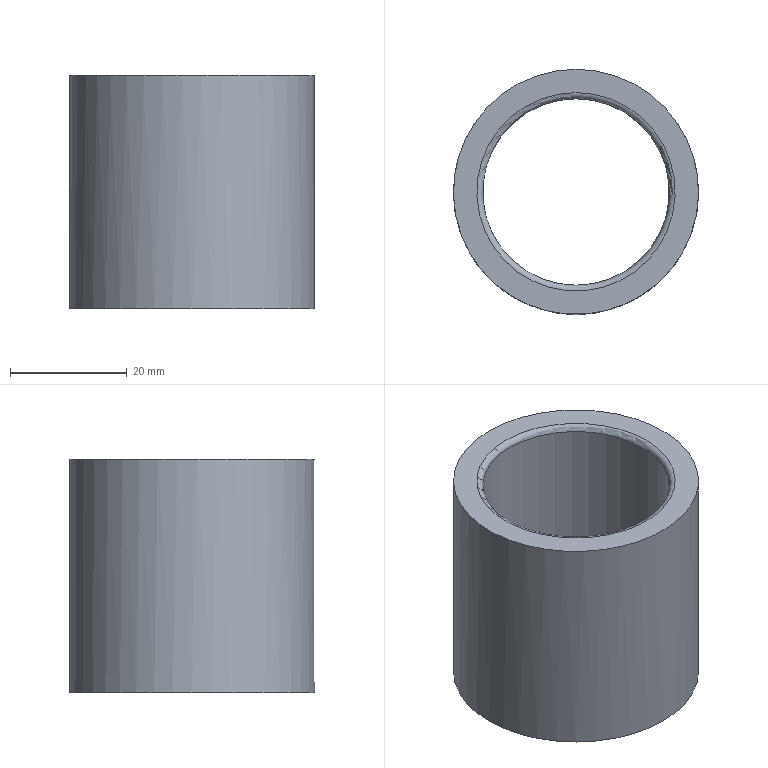Part | STEP file | gslz 2016.10.28-10_id142_x_t | 1 solid | 166 faces | box 42 x 42 x 40 mm | volume 23200 mm3 | other 88 | plane 74 | cylinder 2 | torus 2 | commonest cylinder face diameters 32 x1 42 x1